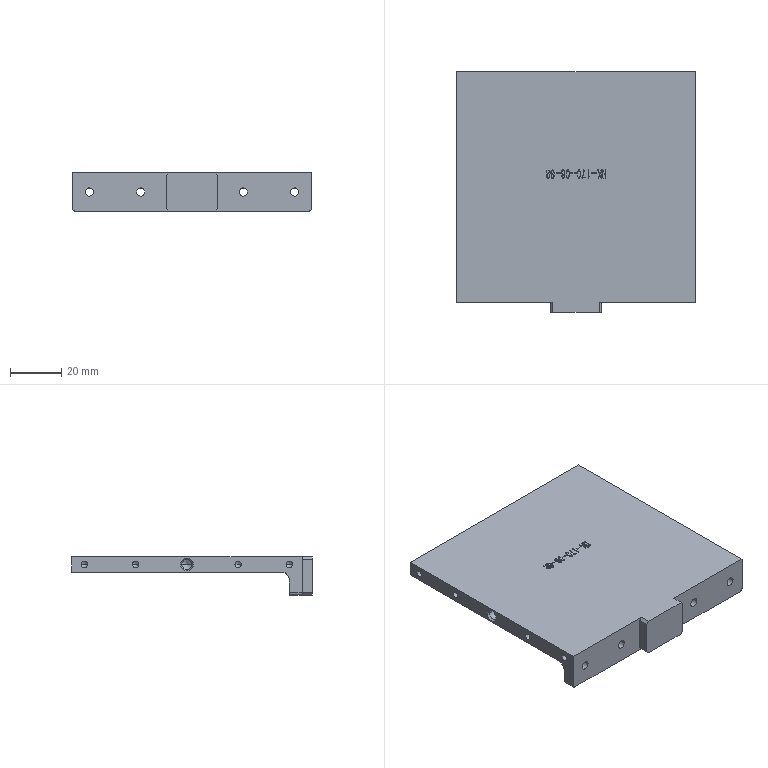NC program | NX | posted with a generic post | part box 93.2 x 94 x 15 mm
Whole program:
N10 G17 G21 G94 G90
(DRILLING_COPY , TOOL : D6A45)
N12 T01 M6
N14 G54
N16 G17 G0 G90 X-40. Y0. B0. C0. S5000 M3
N18 G43 Z30. H1
N20 G94 G81 G98 Z-5.75 F350. R-1.
N22 X-20.
N24 X20.
N26 X40.
N28 G80
N30 G0 X40. Y0. Z30.
N32 M5
(DRILLING_COPY_1_COPY , TOOL : 3.3ZT)
N34 T03 M6
N36 G54
N38 G17 G0 G90 X-40. Y0. B0. C0. S2000 M3
N40 G43 Z30. H3
N42 G94 G83 G98 Z-12.59 F200. Q2. R-1.
N44 X-20.
N46 X20.
N48 X40.
N50 G80
N52 G0 X40. Y0. Z30.
N54 M5
(PLANAR_MILL_COPY_COPY_COPY_COPY_COPY_COPY_1_COPY , TOOL : D6A45)
N56 T01 M6
N58 G54
N60 G17 G0 G90 X-0.866 Y8.9 B0. C0. S9500 M3
N62 G43 Z30. H1
N64 Z0.5
N66 G94 G1 Z-1. F1250.
N68 G3 X0. Y8.4 R1.
N70 G1 X9.
N72 G2 X9.636 Y8.136 R0.9
N74 G1 X10.636 Y7.136
N76 G2 X10.9 Y6.5 R0.9
N78 G1 Y-6.5
N80 G2 X10.636 Y-7.136 R0.9
N82 G1 X9.636 Y-8.136
N84 G2 X9. Y-8.4 R0.9
N86 G1 X-9.
N88 G2 X-9.636 Y-8.136 R0.9
N90 G1 X-10.636 Y-7.136
N92 G2 X-10.9 Y-6.5 R0.9
N94 G1 Y6.5
N96 G2 X-10.636 Y7.136 R0.9
N98 G1 X-9.636 Y8.136
N100 G2 X-9. Y8.4 R0.9
N102 G1 X0.
N104 G3 X0.866 Y8.9 R1.
N106 G1 Z0.5
N108 G0 Z30.
N110 M5
(刀补 , TOOL : D10JING)
N112 T14 M6
N114 G54
N116 G17 G0 G90 X-12.321 Y-13.927 B0. C0. S9500 M3
N118 G43 Z30. H14
N120 Z0.
N122 G94 G1 Z-1. F1000.
N124 G41 X-12.279 Y-13.837 D14
N126 X-11.89 Y-12.389
N128 G3 X-12.148 Y-11.423 R1.
N130 G1 X-12.546 Y-11.025 F1200.
N132 X-13.536 Y-10.036
N134 G2 X-15. Y-6.5 R5.
N136 G1 Y6.5
N138 G2 X-13.536 Y10.036 R5.
N140 G1 X-12.536 Y11.036
N142 X-12.202 Y11.34
N144 X-12.215 Y11.357
N146 X-12.208 Y11.376
N148 X-12.188 Y11.382
N150 X-12.114 Y11.455
N152 G3 X-11.844 Y12.418 R1.
N154 G1 X-12.217 Y13.873
N156 G40
N158 X-12.258 Y13.964
N160 Z0.
N162 G0 Z30.
N164 X-12.323 Y-13.927
N166 Z-1.
N168 G1 Z-2. F1000.
N170 G41 X-12.28 Y-13.836
N172 X-11.891 Y-12.39
N174 G3 X-12.148 Y-11.424 R1.
N176 G1 X-12.546 Y-11.025 F1200.
N178 X-13.536 Y-10.036
N180 G2 X-15. Y-6.5 R5.
N182 G1 Y6.5
N184 G2 X-13.536 Y10.036 R5.
N186 G1 X-12.536 Y11.036
N188 X-12.202 Y11.34
N190 X-12.215 Y11.356
N192 X-12.209 Y11.376
N194 X-12.189 Y11.382
N196 X-12.114 Y11.455
N198 G3 X-11.844 Y12.418 R1.
N200 G1 X-12.217 Y13.873
N202 G40
N204 X-12.258 Y13.964
N206 Z-1.
N208 G0 Z30.
N210 X-12.325 Y-13.926
N212 Z-2.
N214 G1 Z-3. F1000.
N216 G41 X-12.282 Y-13.836
N218 X-11.892 Y-12.391
N220 G3 X-12.149 Y-11.424 R1.
N222 G1 X-12.546 Y-11.025 F1200.
N224 X-13.536 Y-10.036
N226 G2 X-15. Y-6.5 R5.
N228 G1 Y6.5
N230 G2 X-13.536 Y10.036 R5.
N232 G1 X-12.536 Y11.036
N234 X-12.202 Y11.34
N236 X-12.215 Y11.356
N238 X-12.209 Y11.376
N240 X-12.189 Y11.383
N242 X-12.114 Y11.456
N244 G3 X-11.845 Y12.419 R1.
N246 G1 X-12.217 Y13.873
N248 G40
N250 X-12.258 Y13.964
N252 Z-2.
N254 G0 Z30.
N256 X-12.327 Y-13.925
N258 Z-3.
N260 G1 Z-4. F1000.
N262 G41 X-12.284 Y-13.835
N264 X-11.893 Y-12.391
N266 G3 X-12.149 Y-11.424 R1.
N268 G1 X-12.546 Y-11.025 F1200.
N270 X-13.536 Y-10.036
N272 G2 X-15. Y-6.5 R5.
N274 G1 Y6.5
N276 G2 X-13.536 Y10.036 R5.
N278 G1 X-12.536 Y11.036
N280 X-12.217 Y11.328
N282 X-12.216 Y11.356
N284 X-12.121 Y11.449
N286 G3 X-11.86 Y12.415 R1.
N288 G1 X-12.243 Y13.858
N290 G40
N292 X-12.285 Y13.949
N294 Z-3.
N296 G0 Z30.
N298 X12.295 Y13.943
N300 Z0.
N302 G1 Z-1. F1000.
N304 G41 X12.253 Y13.852
N306 X11.871 Y12.401
N308 G3 X12.134 Y11.436 R1.
N310 G1 X12.305 Y11.267 F1200.
N312 X12.311 Y11.246
N314 G2 X12.826 Y10.719 R5.
N316 G1 X12.853 Y10.718
N318 X12.986 Y10.585
N320 X13.536 Y10.036
N322 G2 X15. Y6.5 R5.
N324 G1 Y-6.5
N326 G2 X13.536 Y-10.036 R5.
N328 G1 X12.536 Y-11.036
N330 X12.216 Y-11.328
N332 X12.231 Y-11.342
N334 X12.216 Y-11.355
N336 X12.128 Y-11.443
N338 G3 X11.868 Y-12.409 R1.
N340 G1 X12.253 Y-13.852
N342 G40
N344 X12.295 Y-13.943
N346 Z0.
N348 G0 Z30.
N350 Y13.943
N352 Z-1.
N354 G1 Z-2. F1000.
N356 G41 X12.253 Y13.852
N358 X11.871 Y12.401
N360 G3 X12.134 Y11.437 R1.
N362 G1 X12.305 Y11.267 F1200.
N364 X12.311 Y11.246
N366 G2 X12.826 Y10.719 R5.
N368 G1 X12.853 Y10.718
N370 X12.986 Y10.585
N372 X13.536 Y10.036
N374 G2 X15. Y6.5 R5.
N376 G1 Y-6.5
N378 G2 X13.536 Y-10.036 R5.
N380 G1 X12.536 Y-11.036
N382 X12.216 Y-11.328
N384 X12.231 Y-11.342
N386 X12.216 Y-11.356
N388 X12.128 Y-11.443
N390 G3 X11.868 Y-12.409 R1.
N392 G1 X12.253 Y-13.852
N394 G40
N396 X12.295 Y-13.943
N398 Z-1.
N400 G0 Z30.
N402 X12.298 Y13.941
N404 Z-2.
N406 G1 Z-3. F1000.
N408 G41 X12.256 Y13.851
N410 X11.873 Y12.402
N412 G3 X12.135 Y11.437 R1.
N414 G1 X12.306 Y11.267 F1200.
N416 X12.321 Y11.26
N418 X12.311 Y11.246
N420 G2 X12.826 Y10.719 R5.
N422 G1 X12.854
N424 X12.986 Y10.585
N426 X13.536 Y10.036
N428 G2 X15. Y6.5 R5.
N430 G1 Y-6.5
N432 G2 X13.536 Y-10.036 R5.
N434 G1 X12.546 Y-11.025
N436 X12.536 Y-11.036
N438 X12.216 Y-11.328
N440 X12.232 Y-11.342
N442 X12.216 Y-11.356
N444 X12.128 Y-11.444
N446 G3 X11.868 Y-12.409 R1.
N448 G1 X12.254 Y-13.853
N450 G40
N452 X12.296 Y-13.944
N454 Z-2.
N456 G0 Z30.
N458 X12.3 Y13.941
N460 Z-3.
N462 G1 Z-4. F1000.
N464 G41 X12.258 Y13.85
N466 X11.874 Y12.402
N468 G3 X12.135 Y11.437 R1.
N470 G1 X12.306 Y11.267 F1200.
N472 X12.321 Y11.26
N474 X12.311 Y11.246
N476 G2 X12.826 Y10.719 R5.
N478 G1 X12.854
N480 X12.986 Y10.585
N482 X13.536 Y10.036
N484 G2 X15. Y6.5 R5.
N486 G1 Y-6.5
N488 G2 X13.536 Y-10.036 R5.
N490 G1 X12.546 Y-11.025
N492 X12.537 Y-11.037
N494 X12.231 Y-11.316
N496 X12.245 Y-11.33
N498 X12.23 Y-11.343
N500 X12.135 Y-11.437
N502 G3 X11.876 Y-12.403 R1.
N504 G1 X12.262 Y-13.848
N506 G40
N508 X12.304 Y-13.939
N510 Z-3.
N512 G0 Z30.
N514 M5
N516 M2